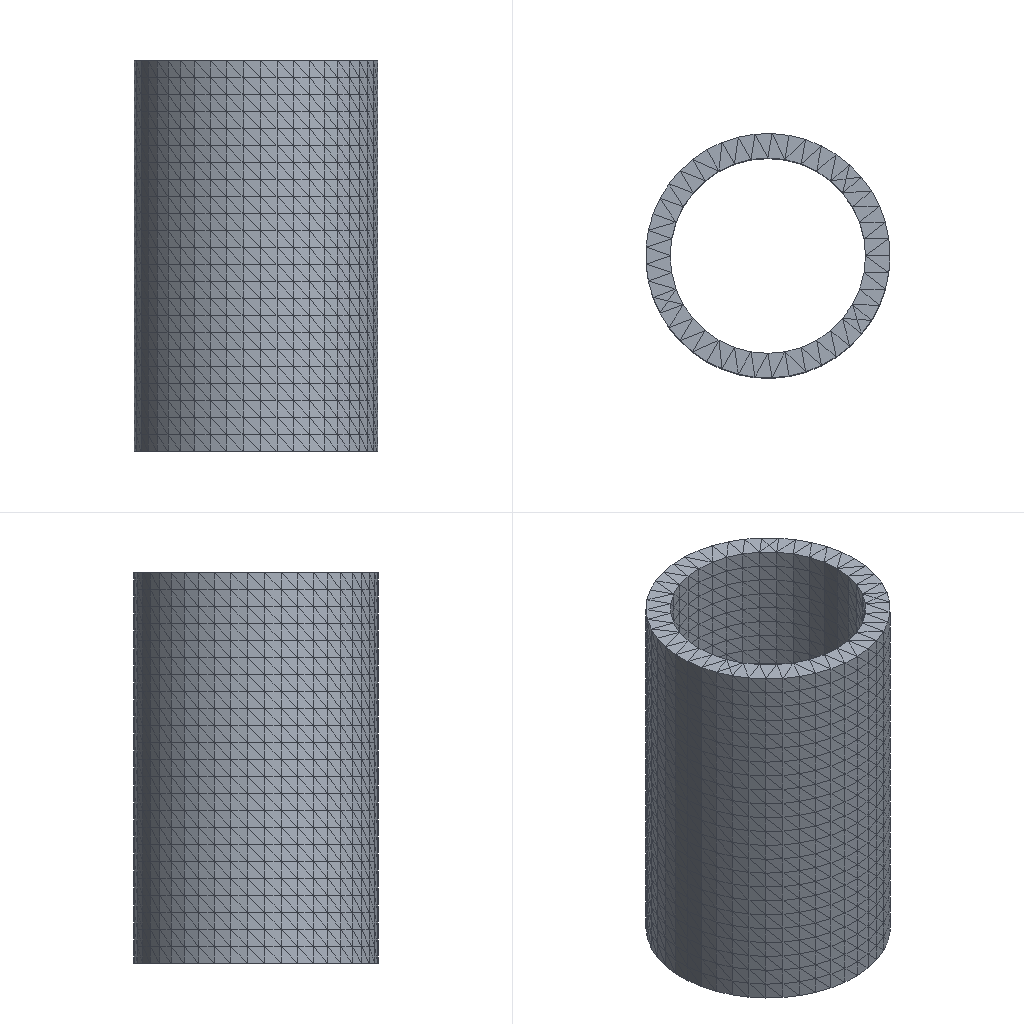Simulation study | abaqus
Notes in the study folder:
06 hollow cylinder
job_status=None
Umax_mm=0.00113657
S_Mises_max_MPa=3.64543
Set-up summary:
category,name,step,type,value,unit,region
solver,abaqus,,Abaqus/CAE 2024
units,mm-N-s-tonne (MPa),,inferred,E=210000 density=7.85e-09
analysis,Step-1,,static,time_period=1
mesh,nodes,,,18200
mesh,elements,,,10686
element_type,C3D10,,,10686
material,Steel,,E,210000
material,Steel,,nu,0.3
material,Steel,,density,7.85e-09
section,Steel,,solid section,,,_PickedSet2
load,Load,Step-1,pressure,3,,LOAD
bc,BC,Step-1,encastre,[dofs=ENCASTRE],,FIXED
Abaqus input file, long lists of numbers shortened:
*Heading
** Job name: deck Model name: M06
** Generated by: Abaqus/CAE 2024
*Preprint, echo=NO, model=NO, history=NO, contact=NO
**
** PARTS
**
*Part, name=P
*Node
      1,          20.,           0.,          80.
      2,          20.,           0.,           0.
** (18198 more lines like these left out)
*Element, type=C3D10
    1,  1951,  1546,  1952,  1590,  2785,  2784,  2783,  2787,  2786,  2788
    2,  1951,  1590,  1953,  1954,  2787,  2790,  2789,  2792,  2791,  2793
** (10684 more lines like these left out)
*Nset, nset=_PickedSet2, internal, generate
     1,  18200,      1
*Elset, elset=_PickedSet2, internal, generate
     1,  10686,      1
** Section: Sec
*Solid Section, elset=_PickedSet2, material=Steel
,
*End Part
**
**
** ASSEMBLY
**
*Assembly, name=Assembly
**
*Instance, name=I, part=P
*End Instance
**
*Nset, nset=FIXED, instance=I
     2,     3,    40,    41,    42,    43,    44,    45,    46,    47,    48,    49,    50,    51,    52,    53
    54,    55,    56,    57,    58,    59,    60,    61,    62,    63,    64,    65,    66,    67,    68,    69
** (14 more lines like these left out)
*Elset, elset=FIXED, instance=I
   12,   28,   29,   30,  107,  109,  110,  145,  151,  168,  173,  319,  321,  340,  419,  493
  494,  572,  946, 1400, 1742, 2003, 2007, 2372, 2420, 2423, 2426, 2557, 2611, 2639, 2640, 2650
** (4 more lines like these left out)
*Elset, elset=_LOAD_S1, internal, instance=I
   26,  203, 3207
*Elset, elset=_LOAD_S3, internal, instance=I
    27,    52,   115,   116,   117,   180,   185,   201,   206,   208,   411,   421,   444,   658,   734,   736
  1220,  1292,  1333,  1404,  1405,  1406,  1418,  1421,  1423,  2544,  2612,  2615,  2641,  2767,  2771,  2911
** (3 more lines like these left out)
*Elset, elset=_LOAD_S4, internal, instance=I
 6465, 6856, 7029, 7144
*Surface, type=ELEMENT, name=LOAD
_LOAD_S1, S1
_LOAD_S3, S3
_LOAD_S4, S4
*End Assembly
**
** MATERIALS
**
*Material, name=Steel
*Density
 7.85e-09,
*Elastic
210000., 0.3
** ----------------------------------------------------------------
**
** STEP: Step-1
**
*Step, name=Step-1, nlgeom=NO
*Static
1., 1., 1e-05, 1.
**
** BOUNDARY CONDITIONS
**
** Name: BC Type: Symmetry/Antisymmetry/Encastre
*Boundary
FIXED, ENCASTRE
**
** LOADS
**
** Name: Load   Type: Pressure
*Dsload
LOAD, P, 3.
**
** OUTPUT REQUESTS
**
*Restart, write, frequency=0
**
** FIELD OUTPUT: F-Output-1
**
*Output, field, variable=PRESELECT
**
** HISTORY OUTPUT: H-Output-1
**
*Output, history, variable=PRESELECT
*End Step
Results summary:
result,odb.job_status,,,JOB_STATUS_COMPLETED_SUCCESSFULLY,"consistent, unstated (Abaqus has no unit system)"
result,steps[0].procedure,Step-1,,*STATIC,"consistent, unstated (Abaqus has no unit system)"
result,steps[0].time_period,Step-1,,1,"consistent, unstated (Abaqus has no unit system)"
result,steps[0].n_frames,Step-1,,2,"consistent, unstated (Abaqus has no unit system)"
result,steps[0].last_frame.id,Step-1,,1,"consistent, unstated (Abaqus has no unit system)"
result,steps[0].last_frame.value,Step-1,,1,"consistent, unstated (Abaqus has no unit system)"
result,steps[0].last_frame.description,Step-1,,Increment      1: Step Time =    1.000,"consistent, unstated (Abaqus has no unit system)"
result,steps[0].completed,Step-1,,True,"consistent, unstated (Abaqus has no unit system)"
result,steps[0].max_U_magnitude,Step-1,,0.001137,"consistent, unstated (Abaqus has no unit system)"
result,steps[0].max_S_mises,Step-1,,3.645,"consistent, unstated (Abaqus has no unit system)"
result,steps[0].RF_sum[1],Step-1,,2.6226e-06,"consistent, unstated (Abaqus has no unit system)"
result,steps[0].RF_sum[2],Step-1,,-3.27826e-06,"consistent, unstated (Abaqus has no unit system)"
result,steps[0].RF_sum[3],Step-1,,2120.58,"consistent, unstated (Abaqus has no unit system)"
result,steps[1].procedure,Step-1,,*STATIC,"consistent, unstated (Abaqus has no unit system)"
result,steps[1].time_period,Step-1,,1,"consistent, unstated (Abaqus has no unit system)"
result,steps[1].n_frames,Step-1,,2,"consistent, unstated (Abaqus has no unit system)"
result,steps[1].last_frame.id,Step-1,,1,"consistent, unstated (Abaqus has no unit system)"
result,steps[1].last_frame.value,Step-1,,1,"consistent, unstated (Abaqus has no unit system)"
result,steps[1].last_frame.description,Step-1,,Increment      1: Step Time =    1.000,"consistent, unstated (Abaqus has no unit system)"
result,steps[1].completed,Step-1,,True,"consistent, unstated (Abaqus has no unit system)"
result,steps[1].max_U_magnitude,Step-1,,0.001137,"consistent, unstated (Abaqus has no unit system)"
result,steps[1].max_S_mises,Step-1,,3.645,"consistent, unstated (Abaqus has no unit system)"
result,steps[1].RF_sum[1],Step-1,,2.6226e-06,"consistent, unstated (Abaqus has no unit system)"
result,steps[1].RF_sum[2],Step-1,,-3.27826e-06,"consistent, unstated (Abaqus has no unit system)"
result,steps[1].RF_sum[3],Step-1,,2120.58,"consistent, unstated (Abaqus has no unit system)"